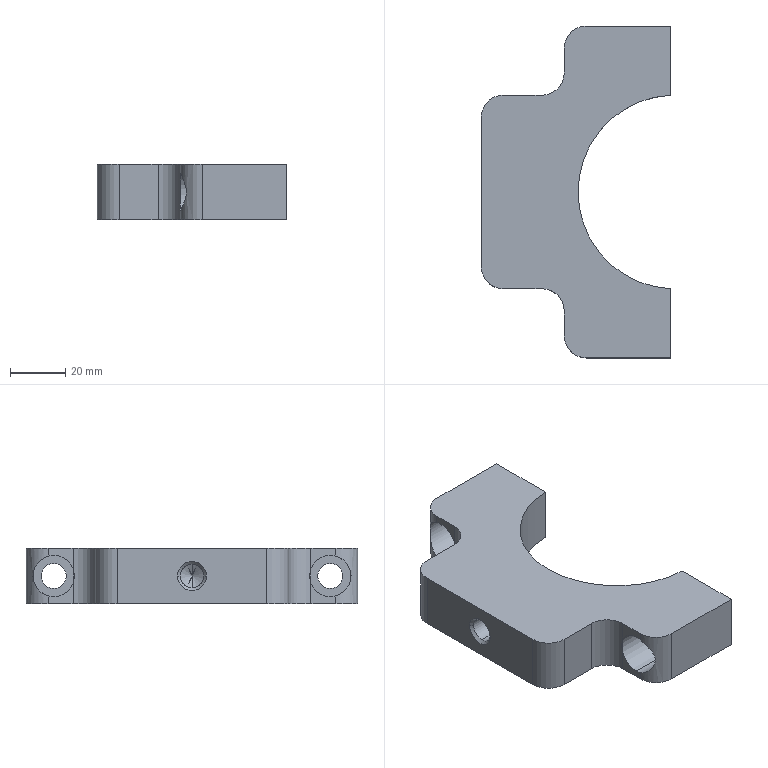Part | STEP file | Handle seat new 2 | 1 solid | 39 faces | box 68.5 x 120 x 20 mm | volume 86648 mm3 | cylinder 18 | plane 17 | cone 4 | commonest cylinder face diameters 16 x6 9 x4 15 x4 8.5 x2 70 x2